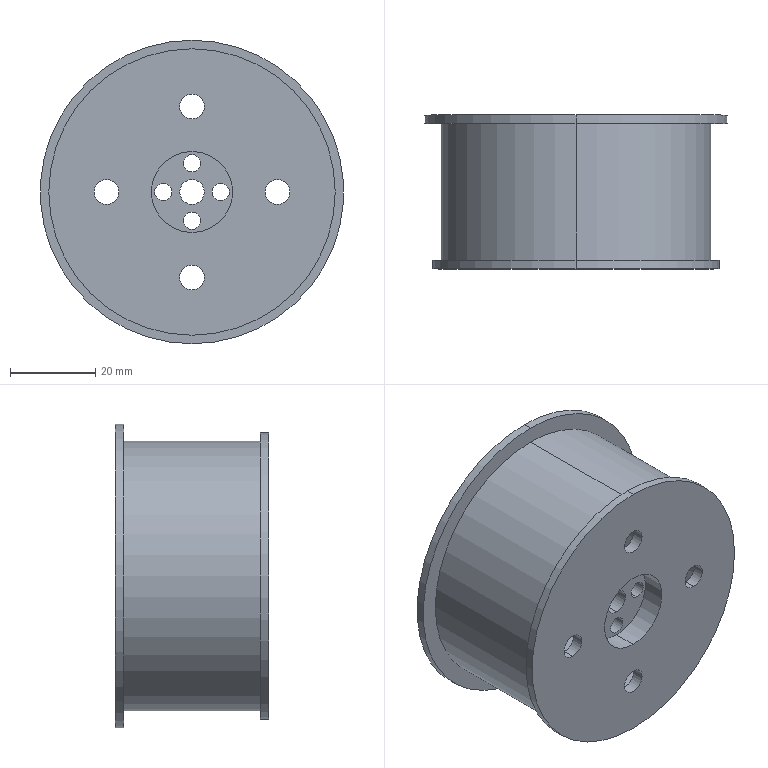Part | STEP file | Polisher large pulley | 1 solid | 40 faces | box 71 x 36 x 71 mm | volume 28167 mm3 | cylinder 32 | plane 8 | commonest cylinder face diameters 5.8 x10 4 x8 19 x2 20 x2 25 x2 58 x2